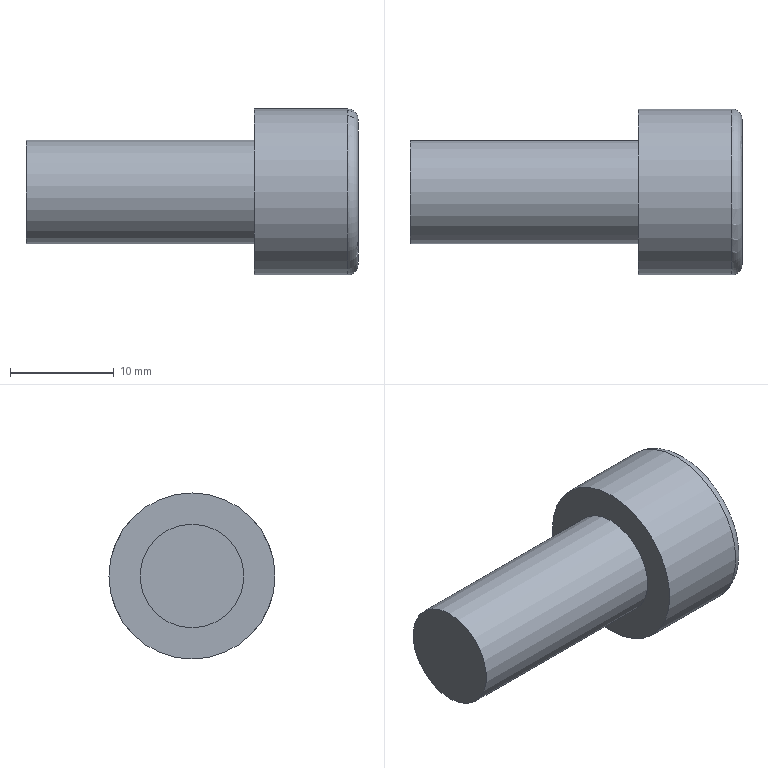Part | STEP file | Tube necking machine_id642_x_t | 1 solid | 13 faces | box 32 x 16 x 16 mm | volume 3362 mm3 | plane 10 | cylinder 2 | torus 1 | commonest cylinder face diameters 10 x1 16 x1
STEP:
#1=CARTESIAN_POINT('',(0.,0.,0.));
#2=DIRECTION('',(0.,0.,1.));
#3=DIRECTION('',(1.,0.,0.));
#4=AXIS2_PLACEMENT_3D('',#1,#2,#3);
#5=CARTESIAN_POINT('',(258.,-103.5,135.5));
#6=VERTEX_POINT('',#5);
#7=CARTESIAN_POINT('',(258.,-103.5,128.5));
#8=DIRECTION('',(1.,0.,0.));
#9=DIRECTION('',(0.,0.,1.));
#10=AXIS2_PLACEMENT_3D('',#7,#8,#9);
#11=CIRCLE('',#10,7.);
#12=CARTESIAN_POINT('',(258.,-103.5,120.5));
#13=DIRECTION('',(-1.,0.,0.));
#14=DIRECTION('',(0.,0.,1.));
#15=AXIS2_PLACEMENT_3D('',#12,#13,#14);
#16=PLANE('',#15);
#17=CARTESIAN_POINT('',(15.,0.));
#18=CARTESIAN_POINT('',(15.,-12.124));
#19=CARTESIAN_POINT('',(4.5,-6.062));
#20=CARTESIAN_POINT('',(-6.,0.));
#21=CARTESIAN_POINT('',(4.5,6.062));
#22=CARTESIAN_POINT('',(15.,12.124));
#23=CARTESIAN_POINT('',(15.,0.));
#24=(BOUNDED_CURVE()B_SPLINE_CURVE(2,(#17,#18,#19,#20,#21,#22,#23),.UNSPECIFIED.,.T.,.F.)B_SPLINE_CURVE_WITH_KNOTS((1,2,2,2,2,1),(-2.094,0.,2.094,4.189,6.283,8.378),.UNSPECIFIED.)CURVE()GEOMETRIC_REPRESENTATION_ITEM()RATIONAL_B_SPLINE_CURVE((1.,0.5,1.,0.5,1.,0.5,1.))REPRESENTATION_ITEM(''));
#25=(GEOMETRIC_REPRESENTATION_CONTEXT(2)PARAMETRIC_REPRESENTATION_CONTEXT()REPRESENTATION_CONTEXT('',''));
#26=DEFINITIONAL_REPRESENTATION('',(#24),#25);
#27=PCURVE('',#16,#26);
#28=CARTESIAN_POINT('',(257.,-103.5,128.5));
#29=DIRECTION('',(-1.,0.,0.));
#30=DIRECTION('',(0.,0.,1.));
#31=AXIS2_PLACEMENT_3D('',#28,#29,#30);
#32=TOROIDAL_SURFACE('',#31,7.,1.);
#33=CARTESIAN_POINT('',(6.283,4.712));
#34=DIRECTION('',(-1.,0.));
#35=VECTOR('',#34,1.);
#36=LINE('',#33,#35);
#37=(GEOMETRIC_REPRESENTATION_CONTEXT(2)PARAMETRIC_REPRESENTATION_CONTEXT()REPRESENTATION_CONTEXT('',''));
#38=DEFINITIONAL_REPRESENTATION('',(#36),#37);
#39=PCURVE('',#32,#38);
#40=SURFACE_CURVE('',#11,(#27,#39),.PCURVE_S1.);
#41=EDGE_CURVE('',#6,#6,#40,.T.);
#42=ORIENTED_EDGE('',*,*,#41,.T.);
#43=EDGE_LOOP('',(#42));
#44=FACE_BOUND('',#43,.T.);
#45=CARTESIAN_POINT('',(258.,-99.5,130.809));
#46=VERTEX_POINT('',#45);
#47=CARTESIAN_POINT('',(258.,-99.5,126.191));
#48=VERTEX_POINT('',#47);
#49=CARTESIAN_POINT('',(258.,-99.5,130.809));
#50=DIRECTION('',(0.,0.,-1.));
#51=VECTOR('',#50,1.);
#52=LINE('',#49,#51);
#53=CARTESIAN_POINT('',(10.309,4.));
#54=DIRECTION('',(-1.,0.));
#55=VECTOR('',#54,1.);
#56=LINE('',#53,#55);
#57=(GEOMETRIC_REPRESENTATION_CONTEXT(2)PARAMETRIC_REPRESENTATION_CONTEXT()REPRESENTATION_CONTEXT('',''));
#58=DEFINITIONAL_REPRESENTATION('',(#56),#57);
#59=PCURVE('',#16,#58);
#60=CARTESIAN_POINT('',(251.4,-99.5,130.809));
#61=DIRECTION('',(0.,-1.,0.));
#62=DIRECTION('',(0.,0.,-1.));
#63=AXIS2_PLACEMENT_3D('',#60,#61,#62);
#64=PLANE('',#63);
#65=CARTESIAN_POINT('',(0.,6.6));
#66=DIRECTION('',(1.,0.));
#67=VECTOR('',#66,1.);
#68=LINE('',#65,#67);
#69=(GEOMETRIC_REPRESENTATION_CONTEXT(2)PARAMETRIC_REPRESENTATION_CONTEXT()REPRESENTATION_CONTEXT('',''));
#70=DEFINITIONAL_REPRESENTATION('',(#68),#69);
#71=PCURVE('',#64,#70);
#72=SURFACE_CURVE('',#52,(#59,#71),.PCURVE_S1.);
#73=EDGE_CURVE('',#46,#48,#72,.T.);
#74=ORIENTED_EDGE('',*,*,#73,.T.);
#75=CARTESIAN_POINT('',(258.,-103.5,123.881));
#76=VERTEX_POINT('',#75);
#77=CARTESIAN_POINT('',(258.,-99.5,126.191));
#78=DIRECTION('',(0.,-0.866,-0.5));
#79=VECTOR('',#78,1.);
#80=LINE('',#77,#79);
#81=CARTESIAN_POINT('',(5.691,4.));
#82=DIRECTION('',(-0.5,-0.866));
#83=VECTOR('',#82,1.);
#84=LINE('',#81,#83);
#85=(GEOMETRIC_REPRESENTATION_CONTEXT(2)PARAMETRIC_REPRESENTATION_CONTEXT()REPRESENTATION_CONTEXT('',''));
#86=DEFINITIONAL_REPRESENTATION('',(#84),#85);
#87=PCURVE('',#16,#86);
#88=CARTESIAN_POINT('',(251.4,-99.5,126.191));
#89=DIRECTION('',(0.,-0.5,0.866));
#90=DIRECTION('',(0.,-0.866,-0.5));
#91=AXIS2_PLACEMENT_3D('',#88,#89,#90);
#92=PLANE('',#91);
#93=CARTESIAN_POINT('',(0.,6.6));
#94=DIRECTION('',(1.,0.));
#95=VECTOR('',#94,1.);
#96=LINE('',#93,#95);
#97=(GEOMETRIC_REPRESENTATION_CONTEXT(2)PARAMETRIC_REPRESENTATION_CONTEXT()REPRESENTATION_CONTEXT('',''));
#98=DEFINITIONAL_REPRESENTATION('',(#96),#97);
#99=PCURVE('',#92,#98);
#100=SURFACE_CURVE('',#80,(#87,#99),.PCURVE_S1.);
#101=EDGE_CURVE('',#48,#76,#100,.T.);
#102=ORIENTED_EDGE('',*,*,#101,.T.);
#103=CARTESIAN_POINT('',(258.,-107.5,126.191));
#104=VERTEX_POINT('',#103);
#105=CARTESIAN_POINT('',(258.,-103.5,123.881));
#106=DIRECTION('',(0.,-0.866,0.5));
#107=VECTOR('',#106,1.);
#108=LINE('',#105,#107);
#109=CARTESIAN_POINT('',(3.381,0.));
#110=DIRECTION('',(0.5,-0.866));
#111=VECTOR('',#110,1.);
#112=LINE('',#109,#111);
#113=(GEOMETRIC_REPRESENTATION_CONTEXT(2)PARAMETRIC_REPRESENTATION_CONTEXT()REPRESENTATION_CONTEXT('',''));
#114=DEFINITIONAL_REPRESENTATION('',(#112),#113);
#115=PCURVE('',#16,#114);
#116=CARTESIAN_POINT('',(251.4,-103.5,123.881));
#117=DIRECTION('',(0.,0.5,0.866));
#118=DIRECTION('',(0.,-0.866,0.5));
#119=AXIS2_PLACEMENT_3D('',#116,#117,#118);
#120=PLANE('',#119);
#121=CARTESIAN_POINT('',(0.,6.6));
#122=DIRECTION('',(1.,0.));
#123=VECTOR('',#122,1.);
#124=LINE('',#121,#123);
#125=(GEOMETRIC_REPRESENTATION_CONTEXT(2)PARAMETRIC_REPRESENTATION_CONTEXT()REPRESENTATION_CONTEXT('',''));
#126=DEFINITIONAL_REPRESENTATION('',(#124),#125);
#127=PCURVE('',#120,#126);
#128=SURFACE_CURVE('',#108,(#115,#127),.PCURVE_S1.);
#129=EDGE_CURVE('',#76,#104,#128,.T.);
#130=ORIENTED_EDGE('',*,*,#129,.T.);
#131=CARTESIAN_POINT('',(258.,-107.5,130.809));
#132=VERTEX_POINT('',#131);
#133=CARTESIAN_POINT('',(258.,-107.5,126.191));
#134=DIRECTION('',(0.,0.,1.));
#135=VECTOR('',#134,1.);
#136=LINE('',#133,#135);
#137=CARTESIAN_POINT('',(5.691,-4.));
#138=DIRECTION('',(1.,0.));
#139=VECTOR('',#138,1.);
#140=LINE('',#137,#139);
#141=(GEOMETRIC_REPRESENTATION_CONTEXT(2)PARAMETRIC_REPRESENTATION_CONTEXT()REPRESENTATION_CONTEXT('',''));
#142=DEFINITIONAL_REPRESENTATION('',(#140),#141);
#143=PCURVE('',#16,#142);
#144=CARTESIAN_POINT('',(251.4,-107.5,126.191));
#145=DIRECTION('',(0.,1.,0.));
#146=DIRECTION('',(0.,0.,1.));
#147=AXIS2_PLACEMENT_3D('',#144,#145,#146);
#148=PLANE('',#147);
#149=CARTESIAN_POINT('',(0.,6.6));
#150=DIRECTION('',(1.,0.));
#151=VECTOR('',#150,1.);
#152=LINE('',#149,#151);
#153=(GEOMETRIC_REPRESENTATION_CONTEXT(2)PARAMETRIC_REPRESENTATION_CONTEXT()REPRESENTATION_CONTEXT('',''));
#154=DEFINITIONAL_REPRESENTATION('',(#152),#153);
#155=PCURVE('',#148,#154);
#156=SURFACE_CURVE('',#136,(#143,#155),.PCURVE_S1.);
#157=EDGE_CURVE('',#104,#132,#156,.T.);
#158=ORIENTED_EDGE('',*,*,#157,.T.);
#159=CARTESIAN_POINT('',(258.,-103.5,133.119));
#160=VERTEX_POINT('',#159);
#161=CARTESIAN_POINT('',(258.,-107.5,130.809));
#162=DIRECTION('',(0.,0.866,0.5));
#163=VECTOR('',#162,1.);
#164=LINE('',#161,#163);
#165=CARTESIAN_POINT('',(10.309,-4.));
#166=DIRECTION('',(0.5,0.866));
#167=VECTOR('',#166,1.);
#168=LINE('',#165,#167);
#169=(GEOMETRIC_REPRESENTATION_CONTEXT(2)PARAMETRIC_REPRESENTATION_CONTEXT()REPRESENTATION_CONTEXT('',''));
#170=DEFINITIONAL_REPRESENTATION('',(#168),#169);
#171=PCURVE('',#16,#170);
#172=CARTESIAN_POINT('',(251.4,-107.5,130.809));
#173=DIRECTION('',(0.,0.5,-0.866));
#174=DIRECTION('',(0.,0.866,0.5));
#175=AXIS2_PLACEMENT_3D('',#172,#173,#174);
#176=PLANE('',#175);
#177=CARTESIAN_POINT('',(0.,6.6));
#178=DIRECTION('',(1.,0.));
#179=VECTOR('',#178,1.);
#180=LINE('',#177,#179);
#181=(GEOMETRIC_REPRESENTATION_CONTEXT(2)PARAMETRIC_REPRESENTATION_CONTEXT()REPRESENTATION_CONTEXT('',''));
#182=DEFINITIONAL_REPRESENTATION('',(#180),#181);
#183=PCURVE('',#176,#182);
#184=SURFACE_CURVE('',#164,(#171,#183),.PCURVE_S1.);
#185=EDGE_CURVE('',#132,#160,#184,.T.);
#186=ORIENTED_EDGE('',*,*,#185,.T.);
#187=CARTESIAN_POINT('',(258.,-103.5,133.119));
#188=DIRECTION('',(0.,0.866,-0.5));
#189=VECTOR('',#188,1.);
#190=LINE('',#187,#189);
#191=CARTESIAN_POINT('',(12.619,0.));
#192=DIRECTION('',(-0.5,0.866));
#193=VECTOR('',#192,1.);
#194=LINE('',#191,#193);
#195=(GEOMETRIC_REPRESENTATION_CONTEXT(2)PARAMETRIC_REPRESENTATION_CONTEXT()REPRESENTATION_CONTEXT('',''));
#196=DEFINITIONAL_REPRESENTATION('',(#194),#195);
#197=PCURVE('',#16,#196);
#198=CARTESIAN_POINT('',(251.4,-103.5,133.119));
#199=DIRECTION('',(0.,-0.5,-0.866));
#200=DIRECTION('',(0.,0.866,-0.5));
#201=AXIS2_PLACEMENT_3D('',#198,#199,#200);
#202=PLANE('',#201);
#203=CARTESIAN_POINT('',(0.,6.6));
#204=DIRECTION('',(1.,0.));
#205=VECTOR('',#204,1.);
#206=LINE('',#203,#205);
#207=(GEOMETRIC_REPRESENTATION_CONTEXT(2)PARAMETRIC_REPRESENTATION_CONTEXT()REPRESENTATION_CONTEXT('',''));
#208=DEFINITIONAL_REPRESENTATION('',(#206),#207);
#209=PCURVE('',#202,#208);
#210=SURFACE_CURVE('',#190,(#197,#209),.PCURVE_S1.);
#211=EDGE_CURVE('',#160,#46,#210,.T.);
#212=ORIENTED_EDGE('',*,*,#211,.T.);
#213=EDGE_LOOP('',(#74,#102,#130,#158,#186,#212));
#214=FACE_BOUND('',#213,.T.);
#215=ADVANCED_FACE('',(#44,#214),#16,.F.);
#216=CARTESIAN_POINT('',(257.,-103.5,136.5));
#217=VERTEX_POINT('',#216);
#218=CARTESIAN_POINT('',(257.,-103.5,120.5));
#219=VERTEX_POINT('',#218);
#220=CARTESIAN_POINT('',(257.,-103.5,128.5));
#221=DIRECTION('',(-1.,0.,0.));
#222=DIRECTION('',(0.,0.,1.));
#223=AXIS2_PLACEMENT_3D('',#220,#221,#222);
#224=CIRCLE('',#223,8.);
#225=CARTESIAN_POINT('',(249.1,-103.5,128.5));
#226=DIRECTION('',(1.,0.,0.));
#227=DIRECTION('',(0.,0.,-1.));
#228=AXIS2_PLACEMENT_3D('',#225,#226,#227);
#229=CYLINDRICAL_SURFACE('',#228,8.);
#230=CARTESIAN_POINT('',(3.142,7.9));
#231=DIRECTION('',(-1.,0.));
#232=VECTOR('',#231,1.);
#233=LINE('',#230,#232);
#234=(GEOMETRIC_REPRESENTATION_CONTEXT(2)PARAMETRIC_REPRESENTATION_CONTEXT()REPRESENTATION_CONTEXT('',''));
#235=DEFINITIONAL_REPRESENTATION('',(#233),#234);
#236=PCURVE('',#229,#235);
#237=CARTESIAN_POINT('',(0.,6.283));
#238=DIRECTION('',(1.,0.));
#239=VECTOR('',#238,1.);
#240=LINE('',#237,#239);
#241=(GEOMETRIC_REPRESENTATION_CONTEXT(2)PARAMETRIC_REPRESENTATION_CONTEXT()REPRESENTATION_CONTEXT('',''));
#242=DEFINITIONAL_REPRESENTATION('',(#240),#241);
#243=PCURVE('',#32,#242);
#244=SURFACE_CURVE('',#224,(#236,#243),.PCURVE_S1.);
#245=EDGE_CURVE('',#217,#219,#244,.T.);
#246=ORIENTED_EDGE('',*,*,#245,.T.);
#247=CARTESIAN_POINT('',(248.,-103.5,120.5));
#248=VERTEX_POINT('',#247);
#249=CARTESIAN_POINT('',(248.,-103.5,120.5));
#250=CARTESIAN_POINT('',(257.,-103.5,120.5));
#251=B_SPLINE_CURVE_WITH_KNOTS('',1,(#249,#250),.UNSPECIFIED.,.F.,.F.,(2,2),(-1.1,7.9),.PIECEWISE_BEZIER_KNOTS.);
#252=CARTESIAN_POINT('',(0.,0.));
#253=DIRECTION('',(0.,1.));
#254=VECTOR('',#253,1.);
#255=LINE('',#252,#254);
#256=(GEOMETRIC_REPRESENTATION_CONTEXT(2)PARAMETRIC_REPRESENTATION_CONTEXT()REPRESENTATION_CONTEXT('',''));
#257=DEFINITIONAL_REPRESENTATION('',(#255),#256);
#258=PCURVE('',#229,#257);
#259=CARTESIAN_POINT('',(6.283,0.));
#260=DIRECTION('',(0.,1.));
#261=VECTOR('',#260,1.);
#262=LINE('',#259,#261);
#263=(GEOMETRIC_REPRESENTATION_CONTEXT(2)PARAMETRIC_REPRESENTATION_CONTEXT()REPRESENTATION_CONTEXT('',''));
#264=DEFINITIONAL_REPRESENTATION('',(#262),#263);
#265=PCURVE('',#229,#264);
#266=SEAM_CURVE('',#251,(#258,#265),.PCURVE_S1.);
#267=EDGE_CURVE('',#248,#219,#266,.T.);
#268=ORIENTED_EDGE('',*,*,#267,.F.);
#269=CARTESIAN_POINT('',(248.,-103.5,128.5));
#270=DIRECTION('',(1.,0.,0.));
#271=DIRECTION('',(0.,0.,-1.));
#272=AXIS2_PLACEMENT_3D('',#269,#270,#271);
#273=CIRCLE('',#272,8.);
#274=CARTESIAN_POINT('',(0.,-1.1));
#275=DIRECTION('',(1.,0.));
#276=VECTOR('',#275,1.);
#277=LINE('',#274,#276);
#278=(GEOMETRIC_REPRESENTATION_CONTEXT(2)PARAMETRIC_REPRESENTATION_CONTEXT()REPRESENTATION_CONTEXT('',''));
#279=DEFINITIONAL_REPRESENTATION('',(#277),#278);
#280=PCURVE('',#229,#279);
#281=CARTESIAN_POINT('',(248.,-103.5,123.5));
#282=DIRECTION('',(1.,0.,0.));
#283=DIRECTION('',(0.,0.,-1.));
#284=AXIS2_PLACEMENT_3D('',#281,#282,#283);
#285=PLANE('',#284);
#286=CARTESIAN_POINT('',(-5.,0.));
#287=DIRECTION('',(1.,0.));
#288=AXIS2_PLACEMENT_2D('',#286,#287);
#289=CIRCLE('',#288,8.);
#290=(GEOMETRIC_REPRESENTATION_CONTEXT(2)PARAMETRIC_REPRESENTATION_CONTEXT()REPRESENTATION_CONTEXT('',''));
#291=DEFINITIONAL_REPRESENTATION('',(#289),#290);
#292=PCURVE('',#285,#291);
#293=SURFACE_CURVE('',#273,(#280,#292),.PCURVE_S1.);
#294=EDGE_CURVE('',#248,#248,#293,.T.);
#295=ORIENTED_EDGE('',*,*,#294,.T.);
#296=ORIENTED_EDGE('',*,*,#267,.T.);
#297=CARTESIAN_POINT('',(257.,-103.5,128.5));
#298=DIRECTION('',(-1.,0.,0.));
#299=DIRECTION('',(0.,0.,1.));
#300=AXIS2_PLACEMENT_3D('',#297,#298,#299);
#301=CIRCLE('',#300,8.);
#302=CARTESIAN_POINT('',(9.425,7.9));
#303=DIRECTION('',(-1.,0.));
#304=VECTOR('',#303,1.);
#305=LINE('',#302,#304);
#306=(GEOMETRIC_REPRESENTATION_CONTEXT(2)PARAMETRIC_REPRESENTATION_CONTEXT()REPRESENTATION_CONTEXT('',''));
#307=DEFINITIONAL_REPRESENTATION('',(#305),#306);
#308=PCURVE('',#229,#307);
#309=CARTESIAN_POINT('',(0.,6.283));
#310=DIRECTION('',(1.,0.));
#311=VECTOR('',#310,1.);
#312=LINE('',#309,#311);
#313=(GEOMETRIC_REPRESENTATION_CONTEXT(2)PARAMETRIC_REPRESENTATION_CONTEXT()REPRESENTATION_CONTEXT('',''));
#314=DEFINITIONAL_REPRESENTATION('',(#312),#313);
#315=PCURVE('',#32,#314);
#316=SURFACE_CURVE('',#301,(#308,#315),.PCURVE_S1.);
#317=EDGE_CURVE('',#219,#217,#316,.T.);
#318=ORIENTED_EDGE('',*,*,#317,.T.);
#319=EDGE_LOOP('',(#246,#268,#295,#296,#318));
#320=FACE_BOUND('',#319,.T.);
#321=ADVANCED_FACE('',(#320),#229,.T.);
#322=ORIENTED_EDGE('',*,*,#294,.F.);
#323=EDGE_LOOP('',(#322));
#324=FACE_BOUND('',#323,.T.);
#325=CARTESIAN_POINT('',(248.,-103.5,123.5));
#326=VERTEX_POINT('',#325);
#327=CARTESIAN_POINT('',(248.,-103.5,128.5));
#328=DIRECTION('',(1.,0.,0.));
#329=DIRECTION('',(0.,0.,-1.));
#330=AXIS2_PLACEMENT_3D('',#327,#328,#329);
#331=CIRCLE('',#330,5.);
#332=CARTESIAN_POINT('',(-5.,0.));
#333=DIRECTION('',(1.,0.));
#334=AXIS2_PLACEMENT_2D('',#332,#333);
#335=CIRCLE('',#334,5.);
#336=(GEOMETRIC_REPRESENTATION_CONTEXT(2)PARAMETRIC_REPRESENTATION_CONTEXT()REPRESENTATION_CONTEXT('',''));
#337=DEFINITIONAL_REPRESENTATION('',(#335),#336);
#338=PCURVE('',#285,#337);
#339=CARTESIAN_POINT('',(249.1,-103.5,128.5));
#340=DIRECTION('',(1.,0.,0.));
#341=DIRECTION('',(0.,0.,-1.));
#342=AXIS2_PLACEMENT_3D('',#339,#340,#341);
#343=CYLINDRICAL_SURFACE('',#342,5.);
#344=CARTESIAN_POINT('',(0.,-1.1));
#345=DIRECTION('',(1.,0.));
#346=VECTOR('',#345,1.);
#347=LINE('',#344,#346);
#348=(GEOMETRIC_REPRESENTATION_CONTEXT(2)PARAMETRIC_REPRESENTATION_CONTEXT()REPRESENTATION_CONTEXT('',''));
#349=DEFINITIONAL_REPRESENTATION('',(#347),#348);
#350=PCURVE('',#343,#349);
#351=SURFACE_CURVE('',#331,(#338,#350),.PCURVE_S1.);
#352=EDGE_CURVE('',#326,#326,#351,.T.);
#353=ORIENTED_EDGE('',*,*,#352,.T.);
#354=EDGE_LOOP('',(#353));
#355=FACE_BOUND('',#354,.T.);
#356=ADVANCED_FACE('',(#324,#355),#285,.F.);
#357=ORIENTED_EDGE('',*,*,#352,.F.);
#358=CARTESIAN_POINT('',(226.,-103.5,123.5));
#359=VERTEX_POINT('',#358);
#360=CARTESIAN_POINT('',(226.,-103.5,123.5));
#361=CARTESIAN_POINT('',(248.,-103.5,123.5));
#362=B_SPLINE_CURVE_WITH_KNOTS('',1,(#360,#361),.UNSPECIFIED.,.F.,.F.,(2,2),(-23.1,-1.1),.PIECEWISE_BEZIER_KNOTS.);
#363=CARTESIAN_POINT('',(0.,0.));
#364=DIRECTION('',(0.,1.));
#365=VECTOR('',#364,1.);
#366=LINE('',#363,#365);
#367=(GEOMETRIC_REPRESENTATION_CONTEXT(2)PARAMETRIC_REPRESENTATION_CONTEXT()REPRESENTATION_CONTEXT('',''));
#368=DEFINITIONAL_REPRESENTATION('',(#366),#367);
#369=PCURVE('',#343,#368);
#370=CARTESIAN_POINT('',(6.283,0.));
#371=DIRECTION('',(0.,1.));
#372=VECTOR('',#371,1.);
#373=LINE('',#370,#372);
#374=(GEOMETRIC_REPRESENTATION_CONTEXT(2)PARAMETRIC_REPRESENTATION_CONTEXT()REPRESENTATION_CONTEXT('',''));
#375=DEFINITIONAL_REPRESENTATION('',(#373),#374);
#376=PCURVE('',#343,#375);
#377=SEAM_CURVE('',#362,(#369,#376),.PCURVE_S1.);
#378=EDGE_CURVE('',#359,#326,#377,.T.);
#379=ORIENTED_EDGE('',*,*,#378,.F.);
#380=CARTESIAN_POINT('',(226.,-103.5,128.5));
#381=DIRECTION('',(1.,0.,0.));
#382=DIRECTION('',(0.,0.,-1.));
#383=AXIS2_PLACEMENT_3D('',#380,#381,#382);
#384=CIRCLE('',#383,5.);
#385=CARTESIAN_POINT('',(0.,-23.1));
#386=DIRECTION('',(1.,0.));
#387=VECTOR('',#386,1.);
#388=LINE('',#385,#387);
#389=(GEOMETRIC_REPRESENTATION_CONTEXT(2)PARAMETRIC_REPRESENTATION_CONTEXT()REPRESENTATION_CONTEXT('',''));
#390=DEFINITIONAL_REPRESENTATION('',(#388),#389);
#391=PCURVE('',#343,#390);
#392=CARTESIAN_POINT('',(226.,-103.5,128.5));
#393=DIRECTION('',(1.,0.,0.));
#394=DIRECTION('',(0.,0.,-1.));
#395=AXIS2_PLACEMENT_3D('',#392,#393,#394);
#396=PLANE('',#395);
#397=CARTESIAN_POINT('',(0.,0.));
#398=DIRECTION('',(1.,0.));
#399=AXIS2_PLACEMENT_2D('',#397,#398);
#400=CIRCLE('',#399,5.);
#401=(GEOMETRIC_REPRESENTATION_CONTEXT(2)PARAMETRIC_REPRESENTATION_CONTEXT()REPRESENTATION_CONTEXT('',''));
#402=DEFINITIONAL_REPRESENTATION('',(#400),#401);
#403=PCURVE('',#396,#402);
#404=SURFACE_CURVE('',#384,(#391,#403),.PCURVE_S1.);
#405=EDGE_CURVE('',#359,#359,#404,.T.);
#406=ORIENTED_EDGE('',*,*,#405,.T.);
#407=ORIENTED_EDGE('',*,*,#378,.T.);
#408=EDGE_LOOP('',(#357,#379,#406,#407));
#409=FACE_BOUND('',#408,.T.);
#410=ADVANCED_FACE('',(#409),#343,.T.);
#411=ORIENTED_EDGE('',*,*,#405,.F.);
#412=EDGE_LOOP('',(#411));
#413=FACE_BOUND('',#412,.T.);
#414=ADVANCED_FACE('',(#413),#396,.F.);
#415=ORIENTED_EDGE('',*,*,#73,.F.);
#416=CARTESIAN_POINT('',(251.4,-99.5,130.809));
#417=VERTEX_POINT('',#416);
#418=CARTESIAN_POINT('',(251.4,-99.5,130.809));
#419=DIRECTION('',(-1.,0.,0.));
#420=VECTOR('',#419,1.);
#421=LINE('',#418,#420);
#422=CARTESIAN_POINT('',(0.,0.));
#423=DIRECTION('',(0.,-1.));
#424=VECTOR('',#423,1.);
#425=LINE('',#422,#424);
#426=(GEOMETRIC_REPRESENTATION_CONTEXT(2)PARAMETRIC_REPRESENTATION_CONTEXT()REPRESENTATION_CONTEXT('',''));
#427=DEFINITIONAL_REPRESENTATION('',(#425),#426);
#428=PCURVE('',#64,#427);
#429=CARTESIAN_POINT('',(4.619,0.));
#430=DIRECTION('',(0.,-1.));
#431=VECTOR('',#430,1.);
#432=LINE('',#429,#431);
#433=(GEOMETRIC_REPRESENTATION_CONTEXT(2)PARAMETRIC_REPRESENTATION_CONTEXT()REPRESENTATION_CONTEXT('',''));
#434=DEFINITIONAL_REPRESENTATION('',(#432),#433);
#435=PCURVE('',#202,#434);
#436=SURFACE_CURVE('',#421,(#428,#435),.PCURVE_S1.);
#437=EDGE_CURVE('',#46,#417,#436,.T.);
#438=ORIENTED_EDGE('',*,*,#437,.T.);
#439=CARTESIAN_POINT('',(251.4,-99.5,126.191));
#440=VERTEX_POINT('',#439);
#441=CARTESIAN_POINT('',(251.4,-99.5,130.809));
#442=DIRECTION('',(0.,0.,1.));
#443=VECTOR('',#442,1.);
#444=LINE('',#441,#443);
#445=CARTESIAN_POINT('',(0.,0.));
#446=DIRECTION('',(-1.,0.));
#447=VECTOR('',#446,1.);
#448=LINE('',#445,#447);
#449=(GEOMETRIC_REPRESENTATION_CONTEXT(2)PARAMETRIC_REPRESENTATION_CONTEXT()REPRESENTATION_CONTEXT('',''));
#450=DEFINITIONAL_REPRESENTATION('',(#448),#449);
#451=PCURVE('',#64,#450);
#452=CARTESIAN_POINT('',(251.4,-103.5,128.5));
#453=DIRECTION('',(-1.,0.,0.));
#454=DIRECTION('',(0.,0.,1.));
#455=AXIS2_PLACEMENT_3D('',#452,#453,#454);
#456=PLANE('',#455);
#457=CARTESIAN_POINT('',(2.309,4.));
#458=DIRECTION('',(1.,0.));
#459=VECTOR('',#458,1.);
#460=LINE('',#457,#459);
#461=(GEOMETRIC_REPRESENTATION_CONTEXT(2)PARAMETRIC_REPRESENTATION_CONTEXT()REPRESENTATION_CONTEXT('',''));
#462=DEFINITIONAL_REPRESENTATION('',(#460),#461);
#463=PCURVE('',#456,#462);
#464=SURFACE_CURVE('',#444,(#451,#463),.PCURVE_S1.);
#465=EDGE_CURVE('',#440,#417,#464,.T.);
#466=ORIENTED_EDGE('',*,*,#465,.F.);
#467=CARTESIAN_POINT('',(251.4,-99.5,126.191));
#468=DIRECTION('',(-1.,0.,0.));
#469=VECTOR('',#468,1.);
#470=LINE('',#467,#469);
#471=CARTESIAN_POINT('',(4.619,0.));
#472=DIRECTION('',(0.,-1.));
#473=VECTOR('',#472,1.);
#474=LINE('',#471,#473);
#475=(GEOMETRIC_REPRESENTATION_CONTEXT(2)PARAMETRIC_REPRESENTATION_CONTEXT()REPRESENTATION_CONTEXT('',''));
#476=DEFINITIONAL_REPRESENTATION('',(#474),#475);
#477=PCURVE('',#64,#476);
#478=CARTESIAN_POINT('',(0.,0.));
#479=DIRECTION('',(0.,-1.));
#480=VECTOR('',#479,1.);
#481=LINE('',#478,#480);
#482=(GEOMETRIC_REPRESENTATION_CONTEXT(2)PARAMETRIC_REPRESENTATION_CONTEXT()REPRESENTATION_CONTEXT('',''));
#483=DEFINITIONAL_REPRESENTATION('',(#481),#482);
#484=PCURVE('',#92,#483);
#485=SURFACE_CURVE('',#470,(#477,#484),.PCURVE_S1.);
#486=EDGE_CURVE('',#48,#440,#485,.T.);
#487=ORIENTED_EDGE('',*,*,#486,.F.);
#488=EDGE_LOOP('',(#415,#438,#466,#487));
#489=FACE_BOUND('',#488,.T.);
#490=ADVANCED_FACE('',(#489),#64,.T.);
#491=ORIENTED_EDGE('',*,*,#101,.F.);
#492=ORIENTED_EDGE('',*,*,#486,.T.);
#493=CARTESIAN_POINT('',(251.4,-103.5,123.881));
#494=VERTEX_POINT('',#493);
#495=CARTESIAN_POINT('',(251.4,-99.5,126.191));
#496=DIRECTION('',(0.,0.866,0.5));
#497=VECTOR('',#496,1.);
#498=LINE('',#495,#497);
#499=CARTESIAN_POINT('',(0.,0.));
#500=DIRECTION('',(-1.,0.));
#501=VECTOR('',#500,1.);
#502=LINE('',#499,#501);
#503=(GEOMETRIC_REPRESENTATION_CONTEXT(2)PARAMETRIC_REPRESENTATION_CONTEXT()REPRESENTATION_CONTEXT('',''));
#504=DEFINITIONAL_REPRESENTATION('',(#502),#503);
#505=PCURVE('',#92,#504);
#506=CARTESIAN_POINT('',(-2.309,4.));
#507=DIRECTION('',(0.5,0.866));
#508=VECTOR('',#507,1.);
#509=LINE('',#506,#508);
#510=(GEOMETRIC_REPRESENTATION_CONTEXT(2)PARAMETRIC_REPRESENTATION_CONTEXT()REPRESENTATION_CONTEXT('',''));
#511=DEFINITIONAL_REPRESENTATION('',(#509),#510);
#512=PCURVE('',#456,#511);
#513=SURFACE_CURVE('',#498,(#505,#512),.PCURVE_S1.);
#514=EDGE_CURVE('',#494,#440,#513,.T.);
#515=ORIENTED_EDGE('',*,*,#514,.F.);
#516=CARTESIAN_POINT('',(251.4,-103.5,123.881));
#517=DIRECTION('',(-1.,0.,0.));
#518=VECTOR('',#517,1.);
#519=LINE('',#516,#518);
#520=CARTESIAN_POINT('',(4.619,0.));
#521=DIRECTION('',(0.,-1.));
#522=VECTOR('',#521,1.);
#523=LINE('',#520,#522);
#524=(GEOMETRIC_REPRESENTATION_CONTEXT(2)PARAMETRIC_REPRESENTATION_CONTEXT()REPRESENTATION_CONTEXT('',''));
#525=DEFINITIONAL_REPRESENTATION('',(#523),#524);
#526=PCURVE('',#92,#525);
#527=CARTESIAN_POINT('',(0.,0.));
#528=DIRECTION('',(0.,-1.));
#529=VECTOR('',#528,1.);
#530=LINE('',#527,#529);
#531=(GEOMETRIC_REPRESENTATION_CONTEXT(2)PARAMETRIC_REPRESENTATION_CONTEXT()REPRESENTATION_CONTEXT('',''));
#532=DEFINITIONAL_REPRESENTATION('',(#530),#531);
#533=PCURVE('',#120,#532);
#534=SURFACE_CURVE('',#519,(#526,#533),.PCURVE_S1.);
#535=EDGE_CURVE('',#76,#494,#534,.T.);
#536=ORIENTED_EDGE('',*,*,#535,.F.);
#537=EDGE_LOOP('',(#491,#492,#515,#536));
#538=FACE_BOUND('',#537,.T.);
#539=ADVANCED_FACE('',(#538),#92,.T.);
#540=ORIENTED_EDGE('',*,*,#129,.F.);
#541=ORIENTED_EDGE('',*,*,#535,.T.);
#542=CARTESIAN_POINT('',(251.4,-107.5,126.191));
#543=VERTEX_POINT('',#542);
#544=CARTESIAN_POINT('',(251.4,-103.5,123.881));
#545=DIRECTION('',(0.,0.866,-0.5));
#546=VECTOR('',#545,1.);
#547=LINE('',#544,#546);
#548=CARTESIAN_POINT('',(0.,0.));
#549=DIRECTION('',(-1.,0.));
#550=VECTOR('',#549,1.);
#551=LINE('',#548,#550);
#552=(GEOMETRIC_REPRESENTATION_CONTEXT(2)PARAMETRIC_REPRESENTATION_CONTEXT()REPRESENTATION_CONTEXT('',''));
#553=DEFINITIONAL_REPRESENTATION('',(#551),#552);
#554=PCURVE('',#120,#553);
#555=CARTESIAN_POINT('',(-4.619,0.));
#556=DIRECTION('',(-0.5,0.866));
#557=VECTOR('',#556,1.);
#558=LINE('',#555,#557);
#559=(GEOMETRIC_REPRESENTATION_CONTEXT(2)PARAMETRIC_REPRESENTATION_CONTEXT()REPRESENTATION_CONTEXT('',''));
#560=DEFINITIONAL_REPRESENTATION('',(#558),#559);
#561=PCURVE('',#456,#560);
#562=SURFACE_CURVE('',#547,(#554,#561),.PCURVE_S1.);
#563=EDGE_CURVE('',#543,#494,#562,.T.);
#564=ORIENTED_EDGE('',*,*,#563,.F.);
#565=CARTESIAN_POINT('',(251.4,-107.5,126.191));
#566=DIRECTION('',(-1.,0.,0.));
#567=VECTOR('',#566,1.);
#568=LINE('',#565,#567);
#569=CARTESIAN_POINT('',(4.619,0.));
#570=DIRECTION('',(0.,-1.));
#571=VECTOR('',#570,1.);
#572=LINE('',#569,#571);
#573=(GEOMETRIC_REPRESENTATION_CONTEXT(2)PARAMETRIC_REPRESENTATION_CONTEXT()REPRESENTATION_CONTEXT('',''));
#574=DEFINITIONAL_REPRESENTATION('',(#572),#573);
#575=PCURVE('',#120,#574);
#576=CARTESIAN_POINT('',(0.,0.));
#577=DIRECTION('',(0.,-1.));
#578=VECTOR('',#577,1.);
#579=LINE('',#576,#578);
#580=(GEOMETRIC_REPRESENTATION_CONTEXT(2)PARAMETRIC_REPRESENTATION_CONTEXT()REPRESENTATION_CONTEXT('',''));
#581=DEFINITIONAL_REPRESENTATION('',(#579),#580);
#582=PCURVE('',#148,#581);
#583=SURFACE_CURVE('',#568,(#575,#582),.PCURVE_S1.);
#584=EDGE_CURVE('',#104,#543,#583,.T.);
#585=ORIENTED_EDGE('',*,*,#584,.F.);
#586=EDGE_LOOP('',(#540,#541,#564,#585));
#587=FACE_BOUND('',#586,.T.);
#588=ADVANCED_FACE('',(#587),#120,.T.);
#589=ORIENTED_EDGE('',*,*,#157,.F.);
#590=ORIENTED_EDGE('',*,*,#584,.T.);
#591=CARTESIAN_POINT('',(251.4,-107.5,130.809));
#592=VERTEX_POINT('',#591);
#593=CARTESIAN_POINT('',(251.4,-107.5,126.191));
#594=DIRECTION('',(0.,0.,-1.));
#595=VECTOR('',#594,1.);
#596=LINE('',#593,#595);
#597=CARTESIAN_POINT('',(0.,0.));
#598=DIRECTION('',(-1.,0.));
#599=VECTOR('',#598,1.);
#600=LINE('',#597,#599);
#601=(GEOMETRIC_REPRESENTATION_CONTEXT(2)PARAMETRIC_REPRESENTATION_CONTEXT()REPRESENTATION_CONTEXT('',''));
#602=DEFINITIONAL_REPRESENTATION('',(#600),#601);
#603=PCURVE('',#148,#602);
#604=CARTESIAN_POINT('',(-2.309,-4.));
#605=DIRECTION('',(-1.,0.));
#606=VECTOR('',#605,1.);
#607=LINE('',#604,#606);
#608=(GEOMETRIC_REPRESENTATION_CONTEXT(2)PARAMETRIC_REPRESENTATION_CONTEXT()REPRESENTATION_CONTEXT('',''));
#609=DEFINITIONAL_REPRESENTATION('',(#607),#608);
#610=PCURVE('',#456,#609);
#611=SURFACE_CURVE('',#596,(#603,#610),.PCURVE_S1.);
#612=EDGE_CURVE('',#592,#543,#611,.T.);
#613=ORIENTED_EDGE('',*,*,#612,.F.);
#614=CARTESIAN_POINT('',(251.4,-107.5,130.809));
#615=DIRECTION('',(-1.,0.,0.));
#616=VECTOR('',#615,1.);
#617=LINE('',#614,#616);
#618=CARTESIAN_POINT('',(4.619,0.));
#619=DIRECTION('',(0.,-1.));
#620=VECTOR('',#619,1.);
#621=LINE('',#618,#620);
#622=(GEOMETRIC_REPRESENTATION_CONTEXT(2)PARAMETRIC_REPRESENTATION_CONTEXT()REPRESENTATION_CONTEXT('',''));
#623=DEFINITIONAL_REPRESENTATION('',(#621),#622);
#624=PCURVE('',#148,#623);
#625=CARTESIAN_POINT('',(0.,0.));
#626=DIRECTION('',(0.,-1.));
#627=VECTOR('',#626,1.);
#628=LINE('',#625,#627);
#629=(GEOMETRIC_REPRESENTATION_CONTEXT(2)PARAMETRIC_REPRESENTATION_CONTEXT()REPRESENTATION_CONTEXT('',''));
#630=DEFINITIONAL_REPRESENTATION('',(#628),#629);
#631=PCURVE('',#176,#630);
#632=SURFACE_CURVE('',#617,(#624,#631),.PCURVE_S1.);
#633=EDGE_CURVE('',#132,#592,#632,.T.);
#634=ORIENTED_EDGE('',*,*,#633,.F.);
#635=EDGE_LOOP('',(#589,#590,#613,#634));
#636=FACE_BOUND('',#635,.T.);
#637=ADVANCED_FACE('',(#636),#148,.T.);
#638=ORIENTED_EDGE('',*,*,#185,.F.);
#639=ORIENTED_EDGE('',*,*,#633,.T.);
#640=CARTESIAN_POINT('',(251.4,-103.5,133.119));
#641=VERTEX_POINT('',#640);
#642=CARTESIAN_POINT('',(251.4,-107.5,130.809));
#643=DIRECTION('',(0.,-0.866,-0.5));
#644=VECTOR('',#643,1.);
#645=LINE('',#642,#644);
#646=CARTESIAN_POINT('',(0.,0.));
#647=DIRECTION('',(-1.,0.));
#648=VECTOR('',#647,1.);
#649=LINE('',#646,#648);
#650=(GEOMETRIC_REPRESENTATION_CONTEXT(2)PARAMETRIC_REPRESENTATION_CONTEXT()REPRESENTATION_CONTEXT('',''));
#651=DEFINITIONAL_REPRESENTATION('',(#649),#650);
#652=PCURVE('',#176,#651);
#653=CARTESIAN_POINT('',(2.309,-4.));
#654=DIRECTION('',(-0.5,-0.866));
#655=VECTOR('',#654,1.);
#656=LINE('',#653,#655);
#657=(GEOMETRIC_REPRESENTATION_CONTEXT(2)PARAMETRIC_REPRESENTATION_CONTEXT()REPRESENTATION_CONTEXT('',''));
#658=DEFINITIONAL_REPRESENTATION('',(#656),#657);
#659=PCURVE('',#456,#658);
#660=SURFACE_CURVE('',#645,(#652,#659),.PCURVE_S1.);
#661=EDGE_CURVE('',#641,#592,#660,.T.);
#662=ORIENTED_EDGE('',*,*,#661,.F.);
#663=CARTESIAN_POINT('',(251.4,-103.5,133.119));
#664=DIRECTION('',(-1.,0.,0.));
#665=VECTOR('',#664,1.);
#666=LINE('',#663,#665);
#667=CARTESIAN_POINT('',(4.619,0.));
#668=DIRECTION('',(0.,-1.));
#669=VECTOR('',#668,1.);
#670=LINE('',#667,#669);
#671=(GEOMETRIC_REPRESENTATION_CONTEXT(2)PARAMETRIC_REPRESENTATION_CONTEXT()REPRESENTATION_CONTEXT('',''));
#672=DEFINITIONAL_REPRESENTATION('',(#670),#671);
#673=PCURVE('',#176,#672);
#674=CARTESIAN_POINT('',(0.,0.));
#675=DIRECTION('',(0.,-1.));
#676=VECTOR('',#675,1.);
#677=LINE('',#674,#676);
#678=(GEOMETRIC_REPRESENTATION_CONTEXT(2)PARAMETRIC_REPRESENTATION_CONTEXT()REPRESENTATION_CONTEXT('',''));
#679=DEFINITIONAL_REPRESENTATION('',(#677),#678);
#680=PCURVE('',#202,#679);
#681=SURFACE_CURVE('',#666,(#673,#680),.PCURVE_S1.);
#682=EDGE_CURVE('',#160,#641,#681,.T.);
#683=ORIENTED_EDGE('',*,*,#682,.F.);
#684=EDGE_LOOP('',(#638,#639,#662,#683));
#685=FACE_BOUND('',#684,.T.);
#686=ADVANCED_FACE('',(#685),#176,.T.);
#687=ORIENTED_EDGE('',*,*,#211,.F.);
#688=ORIENTED_EDGE('',*,*,#682,.T.);
#689=CARTESIAN_POINT('',(251.4,-103.5,133.119));
#690=DIRECTION('',(0.,-0.866,0.5));
#691=VECTOR('',#690,1.);
#692=LINE('',#689,#691);
#693=CARTESIAN_POINT('',(0.,0.));
#694=DIRECTION('',(-1.,0.));
#695=VECTOR('',#694,1.);
#696=LINE('',#693,#695);
#697=(GEOMETRIC_REPRESENTATION_CONTEXT(2)PARAMETRIC_REPRESENTATION_CONTEXT()REPRESENTATION_CONTEXT('',''));
#698=DEFINITIONAL_REPRESENTATION('',(#696),#697);
#699=PCURVE('',#202,#698);
#700=CARTESIAN_POINT('',(4.619,0.));
#701=DIRECTION('',(0.5,-0.866));
#702=VECTOR('',#701,1.);
#703=LINE('',#700,#702);
#704=(GEOMETRIC_REPRESENTATION_CONTEXT(2)PARAMETRIC_REPRESENTATION_CONTEXT()REPRESENTATION_CONTEXT('',''));
#705=DEFINITIONAL_REPRESENTATION('',(#703),#704);
#706=PCURVE('',#456,#705);
#707=SURFACE_CURVE('',#692,(#699,#706),.PCURVE_S1.);
#708=EDGE_CURVE('',#417,#641,#707,.T.);
#709=ORIENTED_EDGE('',*,*,#708,.F.);
#710=ORIENTED_EDGE('',*,*,#437,.F.);
#711=EDGE_LOOP('',(#687,#688,#709,#710));
#712=FACE_BOUND('',#711,.T.);
#713=ADVANCED_FACE('',(#712),#202,.T.);
#714=ORIENTED_EDGE('',*,*,#465,.T.);
#715=ORIENTED_EDGE('',*,*,#708,.T.);
#716=ORIENTED_EDGE('',*,*,#661,.T.);
#717=ORIENTED_EDGE('',*,*,#612,.T.);
#718=ORIENTED_EDGE('',*,*,#563,.T.);
#719=ORIENTED_EDGE('',*,*,#514,.T.);
#720=EDGE_LOOP('',(#714,#715,#716,#717,#718,#719));
#721=FACE_BOUND('',#720,.T.);
#722=ADVANCED_FACE('',(#721),#456,.F.);
#723=ORIENTED_EDGE('',*,*,#245,.F.);
#724=CARTESIAN_POINT('',(258.,-103.5,135.5));
#725=CARTESIAN_POINT('',(258.,-103.5,135.767));
#726=CARTESIAN_POINT('',(257.915,-103.5,136.028));
#727=CARTESIAN_POINT('',(257.752,-103.5,136.252));
#728=CARTESIAN_POINT('',(257.528,-103.5,136.415));
#729=CARTESIAN_POINT('',(257.267,-103.5,136.5));
#730=CARTESIAN_POINT('',(257.,-103.5,136.5));
#731=(BOUNDED_CURVE()B_SPLINE_CURVE(6,(#724,#725,#726,#727,#728,#729,#730),.UNSPECIFIED.,.F.,.F.)B_SPLINE_CURVE_WITH_KNOTS((7,7),(-1.571,0.),.PIECEWISE_BEZIER_KNOTS.)CURVE()GEOMETRIC_REPRESENTATION_ITEM()RATIONAL_B_SPLINE_CURVE((1.031,1.01,0.9979,0.994,0.9979,1.01,1.031))REPRESENTATION_ITEM(''));
#732=CARTESIAN_POINT('',(0.,6.283));
#733=DIRECTION('',(0.,1.));
#734=VECTOR('',#733,1.);
#735=LINE('',#732,#734);
#736=(GEOMETRIC_REPRESENTATION_CONTEXT(2)PARAMETRIC_REPRESENTATION_CONTEXT()REPRESENTATION_CONTEXT('',''));
#737=DEFINITIONAL_REPRESENTATION('',(#735),#736);
#738=PCURVE('',#32,#737);
#739=CARTESIAN_POINT('',(6.283,6.283));
#740=DIRECTION('',(0.,1.));
#741=VECTOR('',#740,1.);
#742=LINE('',#739,#741);
#743=(GEOMETRIC_REPRESENTATION_CONTEXT(2)PARAMETRIC_REPRESENTATION_CONTEXT()REPRESENTATION_CONTEXT('',''));
#744=DEFINITIONAL_REPRESENTATION('',(#742),#743);
#745=PCURVE('',#32,#744);
#746=SEAM_CURVE('',#731,(#738,#745),.PCURVE_S1.);
#747=EDGE_CURVE('',#6,#217,#746,.T.);
#748=ORIENTED_EDGE('',*,*,#747,.F.);
#749=ORIENTED_EDGE('',*,*,#41,.F.);
#750=ORIENTED_EDGE('',*,*,#747,.T.);
#751=ORIENTED_EDGE('',*,*,#317,.F.);
#752=EDGE_LOOP('',(#723,#748,#749,#750,#751));
#753=FACE_BOUND('',#752,.T.);
#754=ADVANCED_FACE('',(#753),#32,.T.);
#755=CLOSED_SHELL('',(#215,#321,#356,#410,#414,#490,#539,#588,#637,#686,#713,#722,#754));
#756=MANIFOLD_SOLID_BREP('',#755);
#757=(LENGTH_UNIT()NAMED_UNIT(*)SI_UNIT(.MILLI.,.METRE.));
#758=UNCERTAINTY_MEASURE_WITH_UNIT(LENGTH_MEASURE(0.000002),#757,'','');
#759=(NAMED_UNIT(*)PLANE_ANGLE_UNIT()SI_UNIT($,.RADIAN.));
#760=(NAMED_UNIT(*)SI_UNIT($,.STERADIAN.)SOLID_ANGLE_UNIT());
#761=(GEOMETRIC_REPRESENTATION_CONTEXT(3)GLOBAL_UNCERTAINTY_ASSIGNED_CONTEXT((#758))GLOBAL_UNIT_ASSIGNED_CONTEXT((#757,#759,#760))REPRESENTATION_CONTEXT('',''));
#762=ADVANCED_BREP_SHAPE_REPRESENTATION('',(#4,#756),#761);